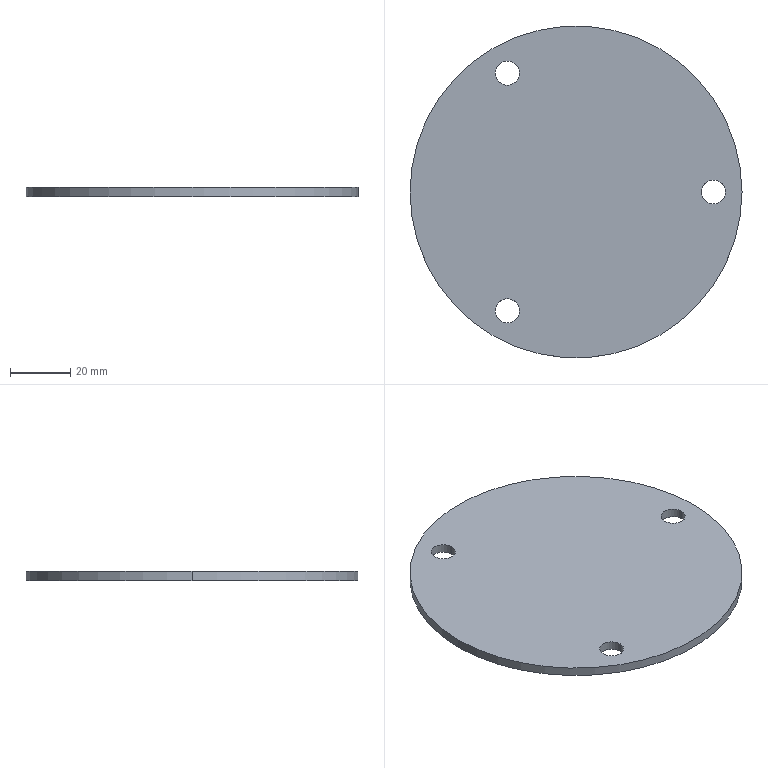Part | SolidWorks | features FlatPattern 1, SMBaseFlange 1, SheetMetal 1 | 1 solid | 10 faces | box 110 x 110 x 3 mm | volume 28058 mm3 | cylinder 8 | plane 2 | commonest cylinder face diameters 8 x6 110 x2
STEP:
#1=CARTESIAN_POINT('',(180.899,260.,3.));
#2=VERTEX_POINT('',#1);
#3=CARTESIAN_POINT('',(188.899,260.,3.));
#4=VERTEX_POINT('',#3);
#5=CARTESIAN_POINT('',(184.899,260.,3.));
#6=DIRECTION('',(0.,0.,1.));
#7=DIRECTION('',(1.,0.,0.));
#8=AXIS2_PLACEMENT_3D('',#5,#6,#7);
#9=CIRCLE('',#8,4.);
#10=EDGE_CURVE('',#2,#4,#9,.T.);
#11=ORIENTED_EDGE('',*,*,#10,.T.);
#12=CARTESIAN_POINT('',(188.899,260.,0.));
#13=VERTEX_POINT('',#12);
#14=CARTESIAN_POINT('',(188.899,260.,3.));
#15=DIRECTION('',(0.,0.,-1.));
#16=VECTOR('',#15,1000.);
#17=LINE('',#14,#16);
#18=EDGE_CURVE('',#4,#13,#17,.T.);
#19=ORIENTED_EDGE('',*,*,#18,.T.);
#20=CARTESIAN_POINT('',(180.899,260.,0.));
#21=VERTEX_POINT('',#20);
#22=CARTESIAN_POINT('',(184.899,260.,0.));
#23=DIRECTION('',(0.,0.,1.));
#24=DIRECTION('',(1.,0.,0.));
#25=AXIS2_PLACEMENT_3D('',#22,#23,#24);
#26=CIRCLE('',#25,4.);
#27=EDGE_CURVE('',#21,#13,#26,.T.);
#28=ORIENTED_EDGE('',*,*,#27,.F.);
#29=CARTESIAN_POINT('',(180.899,260.,3.));
#30=DIRECTION('',(0.,0.,-1.));
#31=VECTOR('',#30,1000.);
#32=LINE('',#29,#31);
#33=EDGE_CURVE('',#2,#21,#32,.T.);
#34=ORIENTED_EDGE('',*,*,#33,.F.);
#35=EDGE_LOOP('',(#11,#19,#28,#34));
#36=FACE_OUTER_BOUND('',#35,.T.);
#37=CARTESIAN_POINT('',(184.899,260.,3.));
#38=DIRECTION('',(0.,0.,-1.));
#39=DIRECTION('',(-1.,0.,0.));
#40=AXIS2_PLACEMENT_3D('',#37,#38,#39);
#41=CYLINDRICAL_SURFACE('',#40,4.);
#42=ADVANCED_FACE('',(#36),#41,.F.);
#43=CARTESIAN_POINT('',(112.649,220.596,3.));
#44=VERTEX_POINT('',#43);
#45=CARTESIAN_POINT('',(120.649,220.596,3.));
#46=VERTEX_POINT('',#45);
#47=CARTESIAN_POINT('',(116.649,220.596,3.));
#48=DIRECTION('',(0.,0.,1.));
#49=DIRECTION('',(1.,0.,0.));
#50=AXIS2_PLACEMENT_3D('',#47,#48,#49);
#51=CIRCLE('',#50,4.);
#52=EDGE_CURVE('',#44,#46,#51,.T.);
#53=ORIENTED_EDGE('',*,*,#52,.T.);
#54=CARTESIAN_POINT('',(120.649,220.596,0.));
#55=VERTEX_POINT('',#54);
#56=CARTESIAN_POINT('',(120.649,220.596,3.));
#57=DIRECTION('',(0.,0.,-1.));
#58=VECTOR('',#57,1000.);
#59=LINE('',#56,#58);
#60=EDGE_CURVE('',#46,#55,#59,.T.);
#61=ORIENTED_EDGE('',*,*,#60,.T.);
#62=CARTESIAN_POINT('',(112.649,220.596,0.));
#63=VERTEX_POINT('',#62);
#64=CARTESIAN_POINT('',(116.649,220.596,0.));
#65=DIRECTION('',(0.,0.,1.));
#66=DIRECTION('',(1.,0.,0.));
#67=AXIS2_PLACEMENT_3D('',#64,#65,#66);
#68=CIRCLE('',#67,4.);
#69=EDGE_CURVE('',#63,#55,#68,.T.);
#70=ORIENTED_EDGE('',*,*,#69,.F.);
#71=CARTESIAN_POINT('',(112.649,220.596,3.));
#72=DIRECTION('',(0.,0.,-1.));
#73=VECTOR('',#72,1000.);
#74=LINE('',#71,#73);
#75=EDGE_CURVE('',#44,#63,#74,.T.);
#76=ORIENTED_EDGE('',*,*,#75,.F.);
#77=EDGE_LOOP('',(#53,#61,#70,#76));
#78=FACE_OUTER_BOUND('',#77,.T.);
#79=CARTESIAN_POINT('',(116.649,220.596,3.));
#80=DIRECTION('',(0.,0.,-1.));
#81=DIRECTION('',(-1.,0.,0.));
#82=AXIS2_PLACEMENT_3D('',#79,#80,#81);
#83=CYLINDRICAL_SURFACE('',#82,4.);
#84=ADVANCED_FACE('',(#78),#83,.F.);
#85=CARTESIAN_POINT('',(112.649,299.404,3.));
#86=VERTEX_POINT('',#85);
#87=CARTESIAN_POINT('',(120.649,299.404,3.));
#88=VERTEX_POINT('',#87);
#89=CARTESIAN_POINT('',(116.649,299.404,3.));
#90=DIRECTION('',(0.,0.,1.));
#91=DIRECTION('',(1.,0.,0.));
#92=AXIS2_PLACEMENT_3D('',#89,#90,#91);
#93=CIRCLE('',#92,4.);
#94=EDGE_CURVE('',#86,#88,#93,.T.);
#95=ORIENTED_EDGE('',*,*,#94,.T.);
#96=CARTESIAN_POINT('',(120.649,299.404,0.));
#97=VERTEX_POINT('',#96);
#98=CARTESIAN_POINT('',(120.649,299.404,3.));
#99=DIRECTION('',(0.,0.,-1.));
#100=VECTOR('',#99,1000.);
#101=LINE('',#98,#100);
#102=EDGE_CURVE('',#88,#97,#101,.T.);
#103=ORIENTED_EDGE('',*,*,#102,.T.);
#104=CARTESIAN_POINT('',(112.649,299.404,0.));
#105=VERTEX_POINT('',#104);
#106=CARTESIAN_POINT('',(116.649,299.404,0.));
#107=DIRECTION('',(0.,0.,1.));
#108=DIRECTION('',(1.,0.,0.));
#109=AXIS2_PLACEMENT_3D('',#106,#107,#108);
#110=CIRCLE('',#109,4.);
#111=EDGE_CURVE('',#105,#97,#110,.T.);
#112=ORIENTED_EDGE('',*,*,#111,.F.);
#113=CARTESIAN_POINT('',(112.649,299.404,3.));
#114=DIRECTION('',(0.,0.,-1.));
#115=VECTOR('',#114,1000.);
#116=LINE('',#113,#115);
#117=EDGE_CURVE('',#86,#105,#116,.T.);
#118=ORIENTED_EDGE('',*,*,#117,.F.);
#119=EDGE_LOOP('',(#95,#103,#112,#118));
#120=FACE_OUTER_BOUND('',#119,.T.);
#121=CARTESIAN_POINT('',(116.649,299.404,3.));
#122=DIRECTION('',(0.,0.,-1.));
#123=DIRECTION('',(-1.,0.,0.));
#124=AXIS2_PLACEMENT_3D('',#121,#122,#123);
#125=CYLINDRICAL_SURFACE('',#124,4.);
#126=ADVANCED_FACE('',(#120),#125,.F.);
#127=CARTESIAN_POINT('',(194.399,260.,3.));
#128=VERTEX_POINT('',#127);
#129=CARTESIAN_POINT('',(84.399,260.,3.));
#130=VERTEX_POINT('',#129);
#131=CARTESIAN_POINT('',(139.399,260.,3.));
#132=DIRECTION('',(0.,0.,1.));
#133=DIRECTION('',(1.,0.,0.));
#134=AXIS2_PLACEMENT_3D('',#131,#132,#133);
#135=CIRCLE('',#134,55.);
#136=EDGE_CURVE('',#128,#130,#135,.T.);
#137=ORIENTED_EDGE('',*,*,#136,.F.);
#138=CARTESIAN_POINT('',(194.399,260.,0.));
#139=VERTEX_POINT('',#138);
#140=CARTESIAN_POINT('',(194.399,260.,3.));
#141=DIRECTION('',(0.,0.,-1.));
#142=VECTOR('',#141,1000.);
#143=LINE('',#140,#142);
#144=EDGE_CURVE('',#128,#139,#143,.T.);
#145=ORIENTED_EDGE('',*,*,#144,.T.);
#146=CARTESIAN_POINT('',(84.399,260.,0.));
#147=VERTEX_POINT('',#146);
#148=CARTESIAN_POINT('',(139.399,260.,0.));
#149=DIRECTION('',(0.,0.,1.));
#150=DIRECTION('',(1.,0.,0.));
#151=AXIS2_PLACEMENT_3D('',#148,#149,#150);
#152=CIRCLE('',#151,55.);
#153=EDGE_CURVE('',#139,#147,#152,.T.);
#154=ORIENTED_EDGE('',*,*,#153,.T.);
#155=CARTESIAN_POINT('',(84.399,260.,3.));
#156=DIRECTION('',(0.,0.,-1.));
#157=VECTOR('',#156,1000.);
#158=LINE('',#155,#157);
#159=EDGE_CURVE('',#130,#147,#158,.T.);
#160=ORIENTED_EDGE('',*,*,#159,.F.);
#161=EDGE_LOOP('',(#137,#145,#154,#160));
#162=FACE_OUTER_BOUND('',#161,.T.);
#163=CARTESIAN_POINT('',(139.399,260.,3.));
#164=DIRECTION('',(0.,0.,-1.));
#165=DIRECTION('',(-1.,0.,0.));
#166=AXIS2_PLACEMENT_3D('',#163,#164,#165);
#167=CYLINDRICAL_SURFACE('',#166,55.);
#168=ADVANCED_FACE('',(#162),#167,.T.);
#169=ORIENTED_EDGE('',*,*,#52,.F.);
#170=CARTESIAN_POINT('',(116.649,220.596,3.));
#171=DIRECTION('',(0.,0.,1.));
#172=DIRECTION('',(1.,0.,0.));
#173=AXIS2_PLACEMENT_3D('',#170,#171,#172);
#174=CIRCLE('',#173,4.);
#175=EDGE_CURVE('',#46,#44,#174,.T.);
#176=ORIENTED_EDGE('',*,*,#175,.F.);
#177=EDGE_LOOP('',(#169,#176));
#178=FACE_BOUND('',#177,.T.);
#179=CARTESIAN_POINT('',(139.399,260.,3.));
#180=DIRECTION('',(0.,0.,1.));
#181=DIRECTION('',(1.,0.,0.));
#182=AXIS2_PLACEMENT_3D('',#179,#180,#181);
#183=CIRCLE('',#182,55.);
#184=EDGE_CURVE('',#130,#128,#183,.T.);
#185=ORIENTED_EDGE('',*,*,#184,.T.);
#186=ORIENTED_EDGE('',*,*,#136,.T.);
#187=EDGE_LOOP('',(#185,#186));
#188=FACE_OUTER_BOUND('',#187,.T.);
#189=ORIENTED_EDGE('',*,*,#94,.F.);
#190=CARTESIAN_POINT('',(116.649,299.404,3.));
#191=DIRECTION('',(0.,0.,1.));
#192=DIRECTION('',(1.,0.,0.));
#193=AXIS2_PLACEMENT_3D('',#190,#191,#192);
#194=CIRCLE('',#193,4.);
#195=EDGE_CURVE('',#88,#86,#194,.T.);
#196=ORIENTED_EDGE('',*,*,#195,.F.);
#197=EDGE_LOOP('',(#189,#196));
#198=FACE_BOUND('',#197,.T.);
#199=ORIENTED_EDGE('',*,*,#10,.F.);
#200=CARTESIAN_POINT('',(184.899,260.,3.));
#201=DIRECTION('',(0.,0.,1.));
#202=DIRECTION('',(1.,0.,0.));
#203=AXIS2_PLACEMENT_3D('',#200,#201,#202);
#204=CIRCLE('',#203,4.);
#205=EDGE_CURVE('',#4,#2,#204,.T.);
#206=ORIENTED_EDGE('',*,*,#205,.F.);
#207=EDGE_LOOP('',(#199,#206));
#208=FACE_BOUND('',#207,.T.);
#209=CARTESIAN_POINT('',(139.399,260.,3.));
#210=DIRECTION('',(0.,0.,1.));
#211=DIRECTION('',(1.,0.,0.));
#212=AXIS2_PLACEMENT_3D('',#209,#210,#211);
#213=PLANE('',#212);
#214=ADVANCED_FACE('',(#178,#188,#198,#208),#213,.T.);
#215=CARTESIAN_POINT('',(139.399,260.,0.));
#216=DIRECTION('',(0.,0.,1.));
#217=DIRECTION('',(1.,0.,0.));
#218=AXIS2_PLACEMENT_3D('',#215,#216,#217);
#219=CIRCLE('',#218,55.);
#220=EDGE_CURVE('',#147,#139,#219,.T.);
#221=ORIENTED_EDGE('',*,*,#220,.F.);
#222=ORIENTED_EDGE('',*,*,#153,.F.);
#223=EDGE_LOOP('',(#221,#222));
#224=FACE_OUTER_BOUND('',#223,.T.);
#225=ORIENTED_EDGE('',*,*,#111,.T.);
#226=CARTESIAN_POINT('',(116.649,299.404,0.));
#227=DIRECTION('',(0.,0.,1.));
#228=DIRECTION('',(1.,0.,0.));
#229=AXIS2_PLACEMENT_3D('',#226,#227,#228);
#230=CIRCLE('',#229,4.);
#231=EDGE_CURVE('',#97,#105,#230,.T.);
#232=ORIENTED_EDGE('',*,*,#231,.T.);
#233=EDGE_LOOP('',(#225,#232));
#234=FACE_BOUND('',#233,.T.);
#235=ORIENTED_EDGE('',*,*,#69,.T.);
#236=CARTESIAN_POINT('',(116.649,220.596,0.));
#237=DIRECTION('',(0.,0.,1.));
#238=DIRECTION('',(1.,0.,0.));
#239=AXIS2_PLACEMENT_3D('',#236,#237,#238);
#240=CIRCLE('',#239,4.);
#241=EDGE_CURVE('',#55,#63,#240,.T.);
#242=ORIENTED_EDGE('',*,*,#241,.T.);
#243=EDGE_LOOP('',(#235,#242));
#244=FACE_BOUND('',#243,.T.);
#245=ORIENTED_EDGE('',*,*,#27,.T.);
#246=CARTESIAN_POINT('',(184.899,260.,0.));
#247=DIRECTION('',(0.,0.,1.));
#248=DIRECTION('',(1.,0.,0.));
#249=AXIS2_PLACEMENT_3D('',#246,#247,#248);
#250=CIRCLE('',#249,4.);
#251=EDGE_CURVE('',#13,#21,#250,.T.);
#252=ORIENTED_EDGE('',*,*,#251,.T.);
#253=EDGE_LOOP('',(#245,#252));
#254=FACE_BOUND('',#253,.T.);
#255=CARTESIAN_POINT('',(139.399,260.,0.));
#256=DIRECTION('',(0.,0.,1.));
#257=DIRECTION('',(1.,0.,0.));
#258=AXIS2_PLACEMENT_3D('',#255,#256,#257);
#259=PLANE('',#258);
#260=ADVANCED_FACE('',(#224,#234,#244,#254),#259,.F.);
#261=ORIENTED_EDGE('',*,*,#144,.F.);
#262=ORIENTED_EDGE('',*,*,#184,.F.);
#263=ORIENTED_EDGE('',*,*,#159,.T.);
#264=ORIENTED_EDGE('',*,*,#220,.T.);
#265=EDGE_LOOP('',(#261,#262,#263,#264));
#266=FACE_OUTER_BOUND('',#265,.T.);
#267=CARTESIAN_POINT('',(139.399,260.,3.));
#268=DIRECTION('',(0.,0.,-1.));
#269=DIRECTION('',(-1.,0.,0.));
#270=AXIS2_PLACEMENT_3D('',#267,#268,#269);
#271=CYLINDRICAL_SURFACE('',#270,55.);
#272=ADVANCED_FACE('',(#266),#271,.T.);
#273=ORIENTED_EDGE('',*,*,#102,.F.);
#274=ORIENTED_EDGE('',*,*,#195,.T.);
#275=ORIENTED_EDGE('',*,*,#117,.T.);
#276=ORIENTED_EDGE('',*,*,#231,.F.);
#277=EDGE_LOOP('',(#273,#274,#275,#276));
#278=FACE_OUTER_BOUND('',#277,.T.);
#279=CARTESIAN_POINT('',(116.649,299.404,3.));
#280=DIRECTION('',(0.,0.,-1.));
#281=DIRECTION('',(-1.,0.,0.));
#282=AXIS2_PLACEMENT_3D('',#279,#280,#281);
#283=CYLINDRICAL_SURFACE('',#282,4.);
#284=ADVANCED_FACE('',(#278),#283,.F.);
#285=ORIENTED_EDGE('',*,*,#60,.F.);
#286=ORIENTED_EDGE('',*,*,#175,.T.);
#287=ORIENTED_EDGE('',*,*,#75,.T.);
#288=ORIENTED_EDGE('',*,*,#241,.F.);
#289=EDGE_LOOP('',(#285,#286,#287,#288));
#290=FACE_OUTER_BOUND('',#289,.T.);
#291=CARTESIAN_POINT('',(116.649,220.596,3.));
#292=DIRECTION('',(0.,0.,-1.));
#293=DIRECTION('',(-1.,0.,0.));
#294=AXIS2_PLACEMENT_3D('',#291,#292,#293);
#295=CYLINDRICAL_SURFACE('',#294,4.);
#296=ADVANCED_FACE('',(#290),#295,.F.);
#297=ORIENTED_EDGE('',*,*,#18,.F.);
#298=ORIENTED_EDGE('',*,*,#205,.T.);
#299=ORIENTED_EDGE('',*,*,#33,.T.);
#300=ORIENTED_EDGE('',*,*,#251,.F.);
#301=EDGE_LOOP('',(#297,#298,#299,#300));
#302=FACE_OUTER_BOUND('',#301,.T.);
#303=CARTESIAN_POINT('',(184.899,260.,3.));
#304=DIRECTION('',(0.,0.,-1.));
#305=DIRECTION('',(-1.,0.,0.));
#306=AXIS2_PLACEMENT_3D('',#303,#304,#305);
#307=CYLINDRICAL_SURFACE('',#306,4.);
#308=ADVANCED_FACE('',(#302),#307,.F.);
#309=CLOSED_SHELL('',(#42,#84,#126,#168,#214,#260,#272,#284,#296,#308));
#310=MANIFOLD_SOLID_BREP('',#309);
#311=CARTESIAN_POINT('',(0.,0.,0.));
#312=DIRECTION('',(0.,0.,1.));
#313=DIRECTION('',(1.,0.,0.));
#314=AXIS2_PLACEMENT_3D('',#311,#312,#313);
#315=(LENGTH_UNIT()NAMED_UNIT(*)SI_UNIT(.MILLI.,.METRE.));
#316=UNCERTAINTY_MEASURE_WITH_UNIT(LENGTH_MEASURE(0.00001),#315,'','');
#317=(NAMED_UNIT(*)PLANE_ANGLE_UNIT()SI_UNIT($,.RADIAN.));
#318=(NAMED_UNIT(*)SI_UNIT($,.STERADIAN.)SOLID_ANGLE_UNIT());
#319=(GEOMETRIC_REPRESENTATION_CONTEXT(3)GLOBAL_UNCERTAINTY_ASSIGNED_CONTEXT((#316))GLOBAL_UNIT_ASSIGNED_CONTEXT((#315,#317,#318))REPRESENTATION_CONTEXT('',''));
#320=ADVANCED_BREP_SHAPE_REPRESENTATION('',(#310,#314),#319);